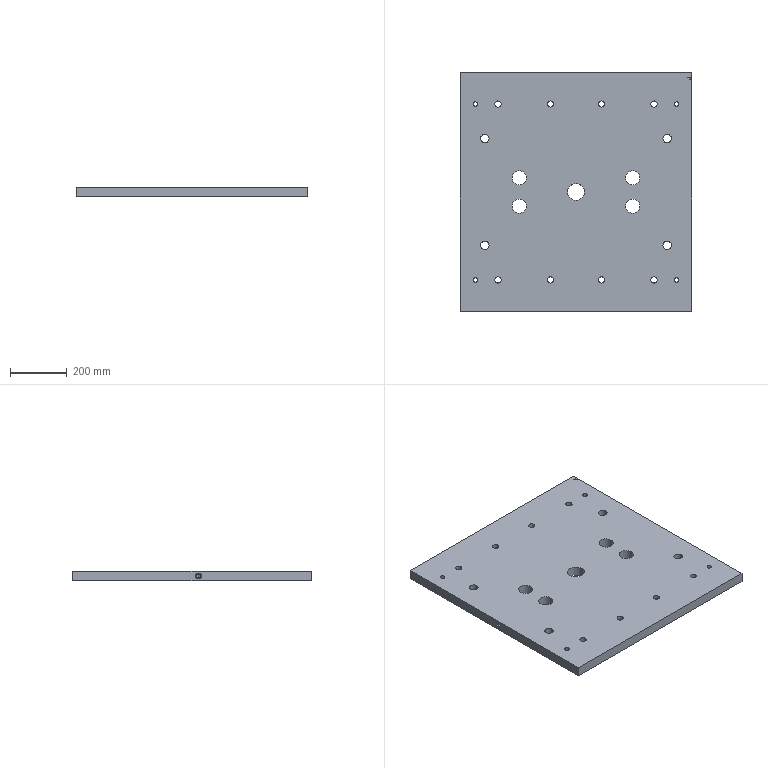Part | Creo | 1 solid | 115 faces | box 815 x 840 x 35 mm | volume 23247158 mm3 | cylinder 78 | plane 29 | cone 8 | commonest cylinder face diameters 22 x16 32 x16 16 x8 23 x8 30 x8 36 x8